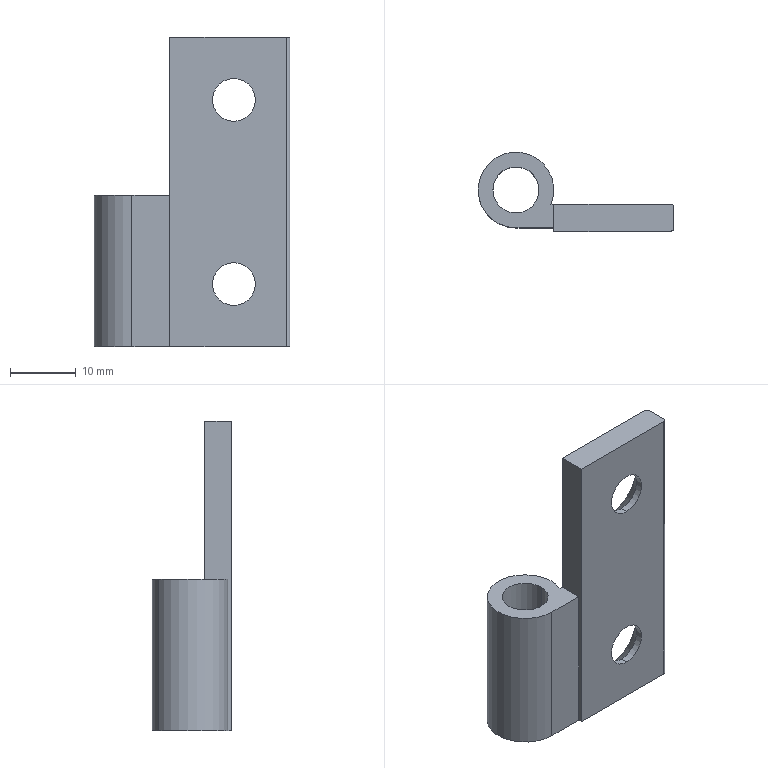Part | SolidWorks | features BaseBody 1 | 1 solid | 22 faces | box 29.75 x 12.05 x 47 mm | volume 4659 mm3 | cylinder 10 | plane 8 | cone 4 | commonest cylinder face diameters 6.5 x4 1 x2 7 x2 11.5 x2
STEP:
#1=CARTESIAN_POINT('',(15.5,1.1,10.75));
#2=VERTEX_POINT('',#1);
#3=CARTESIAN_POINT('',(15.5,1.1,17.25));
#4=VERTEX_POINT('',#3);
#5=CARTESIAN_POINT('',(15.5,1.1,14.));
#6=DIRECTION('',(0.,-1.,0.));
#7=DIRECTION('',(0.,0.,1.));
#8=AXIS2_PLACEMENT_3D('',#5,#6,#7);
#9=CIRCLE('',#8,3.25);
#10=EDGE_CURVE('',#2,#4,#9,.T.);
#11=ORIENTED_EDGE('',*,*,#10,.F.);
#12=CARTESIAN_POINT('',(15.5,0.,10.75));
#13=VERTEX_POINT('',#12);
#14=CARTESIAN_POINT('',(15.5,0.,10.75));
#15=DIRECTION('',(0.,-1.,0.));
#16=VECTOR('',#15,1000.);
#17=LINE('',#14,#16);
#18=EDGE_CURVE('',#2,#13,#17,.T.);
#19=ORIENTED_EDGE('',*,*,#18,.T.);
#20=CARTESIAN_POINT('',(15.5,0.,17.25));
#21=VERTEX_POINT('',#20);
#22=CARTESIAN_POINT('',(15.5,0.,14.));
#23=DIRECTION('',(0.,-1.,0.));
#24=DIRECTION('',(0.,0.,-1.));
#25=AXIS2_PLACEMENT_3D('',#22,#23,#24);
#26=CIRCLE('',#25,3.25);
#27=EDGE_CURVE('',#13,#21,#26,.T.);
#28=ORIENTED_EDGE('',*,*,#27,.T.);
#29=CARTESIAN_POINT('',(15.5,0.,17.25));
#30=DIRECTION('',(0.,-1.,0.));
#31=VECTOR('',#30,1000.);
#32=LINE('',#29,#31);
#33=EDGE_CURVE('',#4,#21,#32,.T.);
#34=ORIENTED_EDGE('',*,*,#33,.F.);
#35=EDGE_LOOP('',(#11,#19,#28,#34));
#36=FACE_OUTER_BOUND('',#35,.T.);
#37=CARTESIAN_POINT('',(15.5,0.,14.));
#38=DIRECTION('',(0.,-1.,0.));
#39=DIRECTION('',(0.000000142,0.,1.));
#40=AXIS2_PLACEMENT_3D('',#37,#38,#39);
#41=CYLINDRICAL_SURFACE('',#40,3.25);
#42=ADVANCED_FACE('',(#36),#41,.F.);
#43=ORIENTED_EDGE('',*,*,#10,.T.);
#44=CARTESIAN_POINT('',(15.5,4.1,20.25));
#45=VERTEX_POINT('',#44);
#46=CARTESIAN_POINT('',(15.5,4.1,20.25));
#47=DIRECTION('',(0.,0.7071,0.7071));
#48=VECTOR('',#47,1000.);
#49=LINE('',#46,#48);
#50=EDGE_CURVE('',#4,#45,#49,.T.);
#51=ORIENTED_EDGE('',*,*,#50,.T.);
#52=CARTESIAN_POINT('',(15.5,4.1,7.75));
#53=VERTEX_POINT('',#52);
#54=CARTESIAN_POINT('',(15.5,4.1,14.));
#55=DIRECTION('',(0.,-1.,0.));
#56=DIRECTION('',(-0.000000001,0.,1.));
#57=AXIS2_PLACEMENT_3D('',#54,#55,#56);
#58=CIRCLE('',#57,6.25);
#59=EDGE_CURVE('',#53,#45,#58,.T.);
#60=ORIENTED_EDGE('',*,*,#59,.F.);
#61=CARTESIAN_POINT('',(15.5,4.1,7.75));
#62=DIRECTION('',(0.,0.7071,-0.7071));
#63=VECTOR('',#62,1000.);
#64=LINE('',#61,#63);
#65=EDGE_CURVE('',#2,#53,#64,.T.);
#66=ORIENTED_EDGE('',*,*,#65,.F.);
#67=EDGE_LOOP('',(#43,#51,#60,#66));
#68=FACE_OUTER_BOUND('',#67,.T.);
#69=CARTESIAN_POINT('',(15.5,4.1,14.));
#70=DIRECTION('',(0.,1.,0.));
#71=DIRECTION('',(0.,0.,-1.));
#72=AXIS2_PLACEMENT_3D('',#69,#70,#71);
#73=CONICAL_SURFACE('',#72,6.25,0.7854);
#74=ADVANCED_FACE('',(#68),#73,.F.);
#75=CARTESIAN_POINT('',(15.5,1.1,-17.25));
#76=VERTEX_POINT('',#75);
#77=CARTESIAN_POINT('',(15.5,1.1,-10.75));
#78=VERTEX_POINT('',#77);
#79=CARTESIAN_POINT('',(15.5,1.1,-14.));
#80=DIRECTION('',(0.,-1.,0.));
#81=DIRECTION('',(0.,0.,1.));
#82=AXIS2_PLACEMENT_3D('',#79,#80,#81);
#83=CIRCLE('',#82,3.25);
#84=EDGE_CURVE('',#76,#78,#83,.T.);
#85=ORIENTED_EDGE('',*,*,#84,.F.);
#86=CARTESIAN_POINT('',(15.5,0.,-17.25));
#87=VERTEX_POINT('',#86);
#88=CARTESIAN_POINT('',(15.5,0.,-17.25));
#89=DIRECTION('',(0.,-1.,0.));
#90=VECTOR('',#89,1000.);
#91=LINE('',#88,#90);
#92=EDGE_CURVE('',#76,#87,#91,.T.);
#93=ORIENTED_EDGE('',*,*,#92,.T.);
#94=CARTESIAN_POINT('',(15.5,0.,-10.75));
#95=VERTEX_POINT('',#94);
#96=CARTESIAN_POINT('',(15.5,0.,-14.));
#97=DIRECTION('',(0.,-1.,0.));
#98=DIRECTION('',(0.,0.,-1.));
#99=AXIS2_PLACEMENT_3D('',#96,#97,#98);
#100=CIRCLE('',#99,3.25);
#101=EDGE_CURVE('',#87,#95,#100,.T.);
#102=ORIENTED_EDGE('',*,*,#101,.T.);
#103=CARTESIAN_POINT('',(15.5,0.,-10.75));
#104=DIRECTION('',(0.,-1.,0.));
#105=VECTOR('',#104,1000.);
#106=LINE('',#103,#105);
#107=EDGE_CURVE('',#78,#95,#106,.T.);
#108=ORIENTED_EDGE('',*,*,#107,.F.);
#109=EDGE_LOOP('',(#85,#93,#102,#108));
#110=FACE_OUTER_BOUND('',#109,.T.);
#111=CARTESIAN_POINT('',(15.5,0.,-14.));
#112=DIRECTION('',(0.,-1.,0.));
#113=DIRECTION('',(0.,0.,1.));
#114=AXIS2_PLACEMENT_3D('',#111,#112,#113);
#115=CYLINDRICAL_SURFACE('',#114,3.25);
#116=ADVANCED_FACE('',(#110),#115,.F.);
#117=ORIENTED_EDGE('',*,*,#84,.T.);
#118=CARTESIAN_POINT('',(15.5,4.1,-7.75));
#119=VERTEX_POINT('',#118);
#120=CARTESIAN_POINT('',(15.5,4.1,-7.75));
#121=DIRECTION('',(0.,0.7071,0.7071));
#122=VECTOR('',#121,1000.);
#123=LINE('',#120,#122);
#124=EDGE_CURVE('',#78,#119,#123,.T.);
#125=ORIENTED_EDGE('',*,*,#124,.T.);
#126=CARTESIAN_POINT('',(15.5,4.1,-20.25));
#127=VERTEX_POINT('',#126);
#128=CARTESIAN_POINT('',(15.5,4.1,-14.));
#129=DIRECTION('',(0.,-1.,0.));
#130=DIRECTION('',(0.,0.,1.));
#131=AXIS2_PLACEMENT_3D('',#128,#129,#130);
#132=CIRCLE('',#131,6.25);
#133=EDGE_CURVE('',#127,#119,#132,.T.);
#134=ORIENTED_EDGE('',*,*,#133,.F.);
#135=CARTESIAN_POINT('',(15.5,4.1,-20.25));
#136=DIRECTION('',(0.,0.7071,-0.7071));
#137=VECTOR('',#136,1000.);
#138=LINE('',#135,#137);
#139=EDGE_CURVE('',#76,#127,#138,.T.);
#140=ORIENTED_EDGE('',*,*,#139,.F.);
#141=EDGE_LOOP('',(#117,#125,#134,#140));
#142=FACE_OUTER_BOUND('',#141,.T.);
#143=CARTESIAN_POINT('',(15.5,4.1,-14.));
#144=DIRECTION('',(0.,1.,0.));
#145=DIRECTION('',(0.,0.,-1.));
#146=AXIS2_PLACEMENT_3D('',#143,#144,#145);
#147=CONICAL_SURFACE('',#146,6.25,0.7854);
#148=ADVANCED_FACE('',(#142),#147,.F.);
#149=CARTESIAN_POINT('',(3.5,6.3,-0.5));
#150=VERTEX_POINT('',#149);
#151=CARTESIAN_POINT('',(-3.5,6.3,-0.5));
#152=VERTEX_POINT('',#151);
#153=CARTESIAN_POINT('',(0.,6.3,-0.5));
#154=DIRECTION('',(0.,0.,1.));
#155=DIRECTION('',(1.,0.,0.));
#156=AXIS2_PLACEMENT_3D('',#153,#154,#155);
#157=CIRCLE('',#156,3.5);
#158=EDGE_CURVE('',#150,#152,#157,.T.);
#159=ORIENTED_EDGE('',*,*,#158,.T.);
#160=CARTESIAN_POINT('',(-3.5,6.3,-23.5));
#161=VERTEX_POINT('',#160);
#162=CARTESIAN_POINT('',(-3.5,6.3,23.5));
#163=DIRECTION('',(0.,0.,-1.));
#164=VECTOR('',#163,1000.);
#165=LINE('',#162,#164);
#166=EDGE_CURVE('',#152,#161,#165,.T.);
#167=ORIENTED_EDGE('',*,*,#166,.T.);
#168=CARTESIAN_POINT('',(3.5,6.3,-23.5));
#169=VERTEX_POINT('',#168);
#170=CARTESIAN_POINT('',(0.,6.3,-23.5));
#171=DIRECTION('',(0.,0.,1.));
#172=DIRECTION('',(-1.,-0.000000142,0.));
#173=AXIS2_PLACEMENT_3D('',#170,#171,#172);
#174=CIRCLE('',#173,3.5);
#175=EDGE_CURVE('',#169,#161,#174,.T.);
#176=ORIENTED_EDGE('',*,*,#175,.F.);
#177=CARTESIAN_POINT('',(3.5,6.3,23.5));
#178=DIRECTION('',(0.,0.,-1.));
#179=VECTOR('',#178,1000.);
#180=LINE('',#177,#179);
#181=EDGE_CURVE('',#150,#169,#180,.T.);
#182=ORIENTED_EDGE('',*,*,#181,.F.);
#183=EDGE_LOOP('',(#159,#167,#176,#182));
#184=FACE_OUTER_BOUND('',#183,.T.);
#185=CARTESIAN_POINT('',(0.,6.3,23.5));
#186=DIRECTION('',(0.,0.,-1.));
#187=DIRECTION('',(1.,0.,0.));
#188=AXIS2_PLACEMENT_3D('',#185,#186,#187);
#189=CYLINDRICAL_SURFACE('',#188,3.5);
#190=ADVANCED_FACE('',(#184),#189,.F.);
#191=CARTESIAN_POINT('',(-3.195,11.081,-0.5));
#192=VERTEX_POINT('',#191);
#193=CARTESIAN_POINT('',(0.,0.55,-0.5));
#194=VERTEX_POINT('',#193);
#195=CARTESIAN_POINT('',(0.,6.3,-0.5));
#196=DIRECTION('',(0.,0.,1.));
#197=DIRECTION('',(0.,-1.,0.));
#198=AXIS2_PLACEMENT_3D('',#195,#196,#197);
#199=CIRCLE('',#198,5.75);
#200=EDGE_CURVE('',#192,#194,#199,.T.);
#201=ORIENTED_EDGE('',*,*,#200,.F.);
#202=CARTESIAN_POINT('',(-3.195,11.081,-23.5));
#203=VERTEX_POINT('',#202);
#204=CARTESIAN_POINT('',(-3.195,11.081,23.5));
#205=DIRECTION('',(0.,0.,-1.));
#206=VECTOR('',#205,1000.);
#207=LINE('',#204,#206);
#208=EDGE_CURVE('',#192,#203,#207,.T.);
#209=ORIENTED_EDGE('',*,*,#208,.T.);
#210=CARTESIAN_POINT('',(0.,0.55,-23.5));
#211=VERTEX_POINT('',#210);
#212=CARTESIAN_POINT('',(0.,6.3,-23.5));
#213=DIRECTION('',(0.,0.,1.));
#214=DIRECTION('',(0.9239,-0.3826,0.));
#215=AXIS2_PLACEMENT_3D('',#212,#213,#214);
#216=CIRCLE('',#215,5.75);
#217=EDGE_CURVE('',#203,#211,#216,.T.);
#218=ORIENTED_EDGE('',*,*,#217,.T.);
#219=CARTESIAN_POINT('',(0.,0.55,-23.5));
#220=DIRECTION('',(0.,0.,-1.));
#221=VECTOR('',#220,1000.);
#222=LINE('',#219,#221);
#223=EDGE_CURVE('',#194,#211,#222,.T.);
#224=ORIENTED_EDGE('',*,*,#223,.F.);
#225=EDGE_LOOP('',(#201,#209,#218,#224));
#226=FACE_OUTER_BOUND('',#225,.T.);
#227=CARTESIAN_POINT('',(0.,6.3,23.5));
#228=DIRECTION('',(0.,0.,-1.));
#229=DIRECTION('',(-0.5556,0.8314,0.));
#230=AXIS2_PLACEMENT_3D('',#227,#228,#229);
#231=CYLINDRICAL_SURFACE('',#230,5.75);
#232=ADVANCED_FACE('',(#226),#231,.T.);
#233=CARTESIAN_POINT('',(5.75,4.1,23.5));
#234=VERTEX_POINT('',#233);
#235=CARTESIAN_POINT('',(5.75,4.1,-0.5));
#236=VERTEX_POINT('',#235);
#237=CARTESIAN_POINT('',(5.75,4.1,-0.5));
#238=DIRECTION('',(0.,0.,-1.));
#239=VECTOR('',#238,1000.);
#240=LINE('',#237,#239);
#241=EDGE_CURVE('',#234,#236,#240,.T.);
#242=ORIENTED_EDGE('',*,*,#241,.F.);
#243=CARTESIAN_POINT('',(23.5,4.1,23.5));
#244=VERTEX_POINT('',#243);
#245=CARTESIAN_POINT('',(5.75,4.1,23.5));
#246=DIRECTION('',(-1.,0.,0.));
#247=VECTOR('',#246,1000.);
#248=LINE('',#245,#247);
#249=EDGE_CURVE('',#244,#234,#248,.T.);
#250=ORIENTED_EDGE('',*,*,#249,.F.);
#251=CARTESIAN_POINT('',(23.5,4.1,-23.5));
#252=VERTEX_POINT('',#251);
#253=CARTESIAN_POINT('',(23.5,4.1,23.5));
#254=DIRECTION('',(0.,0.,-1.));
#255=VECTOR('',#254,1000.);
#256=LINE('',#253,#255);
#257=EDGE_CURVE('',#244,#252,#256,.T.);
#258=ORIENTED_EDGE('',*,*,#257,.T.);
#259=CARTESIAN_POINT('',(5.312,4.1,-23.5));
#260=VERTEX_POINT('',#259);
#261=CARTESIAN_POINT('',(23.5,4.1,-23.5));
#262=DIRECTION('',(-1.,0.,0.));
#263=VECTOR('',#262,1000.);
#264=LINE('',#261,#263);
#265=EDGE_CURVE('',#252,#260,#264,.T.);
#266=ORIENTED_EDGE('',*,*,#265,.T.);
#267=CARTESIAN_POINT('',(5.312,4.1,-0.5));
#268=VERTEX_POINT('',#267);
#269=CARTESIAN_POINT('',(5.312,4.1,-23.5));
#270=DIRECTION('',(0.,0.,-1.));
#271=VECTOR('',#270,1000.);
#272=LINE('',#269,#271);
#273=EDGE_CURVE('',#268,#260,#272,.T.);
#274=ORIENTED_EDGE('',*,*,#273,.F.);
#275=CARTESIAN_POINT('',(5.312,4.1,-0.5));
#276=DIRECTION('',(-1.,0.,0.));
#277=VECTOR('',#276,1000.);
#278=LINE('',#275,#277);
#279=EDGE_CURVE('',#236,#268,#278,.T.);
#280=ORIENTED_EDGE('',*,*,#279,.F.);
#281=EDGE_LOOP('',(#242,#250,#258,#266,#274,#280));
#282=FACE_OUTER_BOUND('',#281,.T.);
#283=ORIENTED_EDGE('',*,*,#133,.T.);
#284=CARTESIAN_POINT('',(15.5,4.1,-14.));
#285=DIRECTION('',(0.,-1.,0.));
#286=DIRECTION('',(0.,0.,1.));
#287=AXIS2_PLACEMENT_3D('',#284,#285,#286);
#288=CIRCLE('',#287,6.25);
#289=EDGE_CURVE('',#119,#127,#288,.T.);
#290=ORIENTED_EDGE('',*,*,#289,.T.);
#291=EDGE_LOOP('',(#283,#290));
#292=FACE_BOUND('',#291,.T.);
#293=ORIENTED_EDGE('',*,*,#59,.T.);
#294=CARTESIAN_POINT('',(15.5,4.1,14.));
#295=DIRECTION('',(0.,-1.,0.));
#296=DIRECTION('',(-0.000000001,0.,1.));
#297=AXIS2_PLACEMENT_3D('',#294,#295,#296);
#298=CIRCLE('',#297,6.25);
#299=EDGE_CURVE('',#45,#53,#298,.T.);
#300=ORIENTED_EDGE('',*,*,#299,.T.);
#301=EDGE_LOOP('',(#293,#300));
#302=FACE_BOUND('',#301,.T.);
#303=CARTESIAN_POINT('',(5.312,4.1,23.5));
#304=DIRECTION('',(0.,1.,0.));
#305=DIRECTION('',(1.,0.,0.));
#306=AXIS2_PLACEMENT_3D('',#303,#304,#305);
#307=PLANE('',#306);
#308=ADVANCED_FACE('',(#282,#292,#302),#307,.T.);
#309=ORIENTED_EDGE('',*,*,#208,.F.);
#310=CARTESIAN_POINT('',(0.,6.3,-0.5));
#311=DIRECTION('',(0.,0.,1.));
#312=DIRECTION('',(0.,-1.,0.));
#313=AXIS2_PLACEMENT_3D('',#310,#311,#312);
#314=CIRCLE('',#313,5.75);
#315=EDGE_CURVE('',#268,#192,#314,.T.);
#316=ORIENTED_EDGE('',*,*,#315,.F.);
#317=ORIENTED_EDGE('',*,*,#273,.T.);
#318=CARTESIAN_POINT('',(0.,6.3,-23.5));
#319=DIRECTION('',(0.,0.,1.));
#320=DIRECTION('',(0.9239,-0.3826,0.));
#321=AXIS2_PLACEMENT_3D('',#318,#319,#320);
#322=CIRCLE('',#321,5.75);
#323=EDGE_CURVE('',#260,#203,#322,.T.);
#324=ORIENTED_EDGE('',*,*,#323,.T.);
#325=EDGE_LOOP('',(#309,#316,#317,#324));
#326=FACE_OUTER_BOUND('',#325,.T.);
#327=CARTESIAN_POINT('',(0.,6.3,23.5));
#328=DIRECTION('',(0.,0.,-1.));
#329=DIRECTION('',(-0.5556,0.8314,0.));
#330=AXIS2_PLACEMENT_3D('',#327,#328,#329);
#331=CYLINDRICAL_SURFACE('',#330,5.75);
#332=ADVANCED_FACE('',(#326),#331,.T.);
#333=CARTESIAN_POINT('',(5.75,0.55,-0.5));
#334=VERTEX_POINT('',#333);
#335=CARTESIAN_POINT('',(5.75,0.55,-0.5));
#336=DIRECTION('',(1.,0.,0.));
#337=VECTOR('',#336,1000.);
#338=LINE('',#335,#337);
#339=EDGE_CURVE('',#194,#334,#338,.T.);
#340=ORIENTED_EDGE('',*,*,#339,.F.);
#341=ORIENTED_EDGE('',*,*,#223,.T.);
#342=CARTESIAN_POINT('',(5.75,0.55,-23.5));
#343=VERTEX_POINT('',#342);
#344=CARTESIAN_POINT('',(0.,0.55,-23.5));
#345=DIRECTION('',(1.,0.,0.));
#346=VECTOR('',#345,1000.);
#347=LINE('',#344,#346);
#348=EDGE_CURVE('',#211,#343,#347,.T.);
#349=ORIENTED_EDGE('',*,*,#348,.T.);
#350=CARTESIAN_POINT('',(5.75,0.55,-23.5));
#351=DIRECTION('',(0.,0.,-1.));
#352=VECTOR('',#351,1000.);
#353=LINE('',#350,#352);
#354=EDGE_CURVE('',#334,#343,#353,.T.);
#355=ORIENTED_EDGE('',*,*,#354,.F.);
#356=EDGE_LOOP('',(#340,#341,#349,#355));
#357=FACE_OUTER_BOUND('',#356,.T.);
#358=CARTESIAN_POINT('',(0.,0.55,-23.5));
#359=DIRECTION('',(0.,-1.,0.));
#360=DIRECTION('',(1.,0.,0.));
#361=AXIS2_PLACEMENT_3D('',#358,#359,#360);
#362=PLANE('',#361);
#363=ADVANCED_FACE('',(#357),#362,.T.);
#364=ORIENTED_EDGE('',*,*,#249,.T.);
#365=CARTESIAN_POINT('',(5.75,0.,23.5));
#366=VERTEX_POINT('',#365);
#367=CARTESIAN_POINT('',(5.75,4.1,23.5));
#368=DIRECTION('',(0.,-1.,0.));
#369=VECTOR('',#368,1000.);
#370=LINE('',#367,#369);
#371=EDGE_CURVE('',#234,#366,#370,.T.);
#372=ORIENTED_EDGE('',*,*,#371,.T.);
#373=CARTESIAN_POINT('',(23.5,0.,23.5));
#374=VERTEX_POINT('',#373);
#375=CARTESIAN_POINT('',(5.75,0.,23.5));
#376=DIRECTION('',(1.,0.,0.));
#377=VECTOR('',#376,1000.);
#378=LINE('',#375,#377);
#379=EDGE_CURVE('',#366,#374,#378,.T.);
#380=ORIENTED_EDGE('',*,*,#379,.T.);
#381=CARTESIAN_POINT('',(24.,0.5,23.5));
#382=VERTEX_POINT('',#381);
#383=CARTESIAN_POINT('',(23.5,0.5,23.5));
#384=DIRECTION('',(0.,0.,1.));
#385=DIRECTION('',(0.,-1.,0.));
#386=AXIS2_PLACEMENT_3D('',#383,#384,#385);
#387=CIRCLE('',#386,0.5);
#388=EDGE_CURVE('',#374,#382,#387,.T.);
#389=ORIENTED_EDGE('',*,*,#388,.T.);
#390=CARTESIAN_POINT('',(24.,3.6,23.5));
#391=VERTEX_POINT('',#390);
#392=CARTESIAN_POINT('',(24.,0.5,23.5));
#393=DIRECTION('',(0.,1.,0.));
#394=VECTOR('',#393,1000.);
#395=LINE('',#392,#394);
#396=EDGE_CURVE('',#382,#391,#395,.T.);
#397=ORIENTED_EDGE('',*,*,#396,.T.);
#398=CARTESIAN_POINT('',(23.5,3.6,23.5));
#399=DIRECTION('',(0.,0.,1.));
#400=DIRECTION('',(1.,0.,0.));
#401=AXIS2_PLACEMENT_3D('',#398,#399,#400);
#402=CIRCLE('',#401,0.5);
#403=EDGE_CURVE('',#391,#244,#402,.T.);
#404=ORIENTED_EDGE('',*,*,#403,.T.);
#405=EDGE_LOOP('',(#364,#372,#380,#389,#397,#404));
#406=FACE_OUTER_BOUND('',#405,.T.);
#407=CARTESIAN_POINT('',(5.75,0.,23.5));
#408=DIRECTION('',(0.,0.,1.));
#409=DIRECTION('',(1.,0.,0.));
#410=AXIS2_PLACEMENT_3D('',#407,#408,#409);
#411=PLANE('',#410);
#412=ADVANCED_FACE('',(#406),#411,.T.);
#413=ORIENTED_EDGE('',*,*,#371,.F.);
#414=ORIENTED_EDGE('',*,*,#241,.T.);
#415=CARTESIAN_POINT('',(5.75,4.1,-0.5));
#416=DIRECTION('',(0.,-1.,0.));
#417=VECTOR('',#416,1000.);
#418=LINE('',#415,#417);
#419=EDGE_CURVE('',#236,#334,#418,.T.);
#420=ORIENTED_EDGE('',*,*,#419,.T.);
#421=ORIENTED_EDGE('',*,*,#354,.T.);
#422=CARTESIAN_POINT('',(5.75,0.,-23.5));
#423=VERTEX_POINT('',#422);
#424=CARTESIAN_POINT('',(5.75,0.55,-23.5));
#425=DIRECTION('',(0.,-1.,0.));
#426=VECTOR('',#425,1000.);
#427=LINE('',#424,#426);
#428=EDGE_CURVE('',#343,#423,#427,.T.);
#429=ORIENTED_EDGE('',*,*,#428,.T.);
#430=CARTESIAN_POINT('',(5.75,0.,-23.5));
#431=DIRECTION('',(0.,0.,-1.));
#432=VECTOR('',#431,1000.);
#433=LINE('',#430,#432);
#434=EDGE_CURVE('',#366,#423,#433,.T.);
#435=ORIENTED_EDGE('',*,*,#434,.F.);
#436=EDGE_LOOP('',(#413,#414,#420,#421,#429,#435));
#437=FACE_OUTER_BOUND('',#436,.T.);
#438=CARTESIAN_POINT('',(5.75,0.,23.5));
#439=DIRECTION('',(-1.,0.,0.));
#440=DIRECTION('',(0.,1.,0.));
#441=AXIS2_PLACEMENT_3D('',#438,#439,#440);
#442=PLANE('',#441);
#443=ADVANCED_FACE('',(#437),#442,.T.);
#444=CARTESIAN_POINT('',(23.5,0.,-23.5));
#445=VERTEX_POINT('',#444);
#446=CARTESIAN_POINT('',(5.75,0.,-23.5));
#447=DIRECTION('',(1.,0.,0.));
#448=VECTOR('',#447,1000.);
#449=LINE('',#446,#448);
#450=EDGE_CURVE('',#423,#445,#449,.T.);
#451=ORIENTED_EDGE('',*,*,#450,.T.);
#452=CARTESIAN_POINT('',(23.5,0.,-23.5));
#453=DIRECTION('',(0.,0.,-1.));
#454=VECTOR('',#453,1000.);
#455=LINE('',#452,#454);
#456=EDGE_CURVE('',#374,#445,#455,.T.);
#457=ORIENTED_EDGE('',*,*,#456,.F.);
#458=ORIENTED_EDGE('',*,*,#379,.F.);
#459=ORIENTED_EDGE('',*,*,#434,.T.);
#460=EDGE_LOOP('',(#451,#457,#458,#459));
#461=FACE_OUTER_BOUND('',#460,.T.);
#462=CARTESIAN_POINT('',(15.5,0.,-14.));
#463=DIRECTION('',(0.,-1.,0.));
#464=DIRECTION('',(0.,0.,-1.));
#465=AXIS2_PLACEMENT_3D('',#462,#463,#464);
#466=CIRCLE('',#465,3.25);
#467=EDGE_CURVE('',#95,#87,#466,.T.);
#468=ORIENTED_EDGE('',*,*,#467,.F.);
#469=ORIENTED_EDGE('',*,*,#101,.F.);
#470=EDGE_LOOP('',(#468,#469));
#471=FACE_BOUND('',#470,.T.);
#472=CARTESIAN_POINT('',(15.5,0.,14.));
#473=DIRECTION('',(0.,-1.,0.));
#474=DIRECTION('',(0.,0.,-1.));
#475=AXIS2_PLACEMENT_3D('',#472,#473,#474);
#476=CIRCLE('',#475,3.25);
#477=EDGE_CURVE('',#21,#13,#476,.T.);
#478=ORIENTED_EDGE('',*,*,#477,.F.);
#479=ORIENTED_EDGE('',*,*,#27,.F.);
#480=EDGE_LOOP('',(#478,#479));
#481=FACE_BOUND('',#480,.T.);
#482=CARTESIAN_POINT('',(5.75,0.,-23.5));
#483=DIRECTION('',(0.,-1.,0.));
#484=DIRECTION('',(1.,0.,0.));
#485=AXIS2_PLACEMENT_3D('',#482,#483,#484);
#486=PLANE('',#485);
#487=ADVANCED_FACE('',(#461,#471,#481),#486,.T.);
#488=CARTESIAN_POINT('',(24.,0.5,-23.5));
#489=VERTEX_POINT('',#488);
#490=CARTESIAN_POINT('',(23.5,0.5,-23.5));
#491=DIRECTION('',(0.,0.,1.));
#492=DIRECTION('',(0.,-1.,0.));
#493=AXIS2_PLACEMENT_3D('',#490,#491,#492);
#494=CIRCLE('',#493,0.5);
#495=EDGE_CURVE('',#445,#489,#494,.T.);
#496=ORIENTED_EDGE('',*,*,#495,.T.);
#497=CARTESIAN_POINT('',(24.,0.5,-23.5));
#498=DIRECTION('',(0.,0.,-1.));
#499=VECTOR('',#498,1000.);
#500=LINE('',#497,#499);
#501=EDGE_CURVE('',#382,#489,#500,.T.);
#502=ORIENTED_EDGE('',*,*,#501,.F.);
#503=ORIENTED_EDGE('',*,*,#388,.F.);
#504=ORIENTED_EDGE('',*,*,#456,.T.);
#505=EDGE_LOOP('',(#496,#502,#503,#504));
#506=FACE_OUTER_BOUND('',#505,.T.);
#507=CARTESIAN_POINT('',(23.5,0.5,23.5));
#508=DIRECTION('',(0.,0.,-1.));
#509=DIRECTION('',(1.,0.,0.));
#510=AXIS2_PLACEMENT_3D('',#507,#508,#509);
#511=CYLINDRICAL_SURFACE('',#510,0.5);
#512=ADVANCED_FACE('',(#506),#511,.T.);
#513=CARTESIAN_POINT('',(24.,3.6,-23.5));
#514=VERTEX_POINT('',#513);
#515=CARTESIAN_POINT('',(24.,0.5,-23.5));
#516=DIRECTION('',(0.,1.,0.));
#517=VECTOR('',#516,1000.);
#518=LINE('',#515,#517);
#519=EDGE_CURVE('',#489,#514,#518,.T.);
#520=ORIENTED_EDGE('',*,*,#519,.T.);
#521=CARTESIAN_POINT('',(24.,3.6,-23.5));
#522=DIRECTION('',(0.,0.,-1.));
#523=VECTOR('',#522,1000.);
#524=LINE('',#521,#523);
#525=EDGE_CURVE('',#391,#514,#524,.T.);
#526=ORIENTED_EDGE('',*,*,#525,.F.);
#527=ORIENTED_EDGE('',*,*,#396,.F.);
#528=ORIENTED_EDGE('',*,*,#501,.T.);
#529=EDGE_LOOP('',(#520,#526,#527,#528));
#530=FACE_OUTER_BOUND('',#529,.T.);
#531=CARTESIAN_POINT('',(24.,0.5,-23.5));
#532=DIRECTION('',(1.,0.,0.));
#533=DIRECTION('',(0.,1.,0.));
#534=AXIS2_PLACEMENT_3D('',#531,#532,#533);
#535=PLANE('',#534);
#536=ADVANCED_FACE('',(#530),#535,.T.);
#537=CARTESIAN_POINT('',(23.5,3.6,-23.5));
#538=DIRECTION('',(0.,0.,1.));
#539=DIRECTION('',(1.,0.,0.));
#540=AXIS2_PLACEMENT_3D('',#537,#538,#539);
#541=CIRCLE('',#540,0.5);
#542=EDGE_CURVE('',#514,#252,#541,.T.);
#543=ORIENTED_EDGE('',*,*,#542,.T.);
#544=ORIENTED_EDGE('',*,*,#257,.F.);
#545=ORIENTED_EDGE('',*,*,#403,.F.);
#546=ORIENTED_EDGE('',*,*,#525,.T.);
#547=EDGE_LOOP('',(#543,#544,#545,#546));
#548=FACE_OUTER_BOUND('',#547,.T.);
#549=CARTESIAN_POINT('',(23.5,3.6,23.5));
#550=DIRECTION('',(0.,0.,-1.));
#551=DIRECTION('',(0.,1.,0.));
#552=AXIS2_PLACEMENT_3D('',#549,#550,#551);
#553=CYLINDRICAL_SURFACE('',#552,0.5);
#554=ADVANCED_FACE('',(#548),#553,.T.);
#555=ORIENTED_EDGE('',*,*,#323,.F.);
#556=ORIENTED_EDGE('',*,*,#265,.F.);
#557=ORIENTED_EDGE('',*,*,#542,.F.);
#558=ORIENTED_EDGE('',*,*,#519,.F.);
#559=ORIENTED_EDGE('',*,*,#495,.F.);
#560=ORIENTED_EDGE('',*,*,#450,.F.);
#561=ORIENTED_EDGE('',*,*,#428,.F.);
#562=ORIENTED_EDGE('',*,*,#348,.F.);
#563=ORIENTED_EDGE('',*,*,#217,.F.);
#564=EDGE_LOOP('',(#555,#556,#557,#558,#559,#560,#561,#562,#563));
#565=FACE_OUTER_BOUND('',#564,.T.);
#566=ORIENTED_EDGE('',*,*,#175,.T.);
#567=CARTESIAN_POINT('',(0.,6.3,-23.5));
#568=DIRECTION('',(0.,0.,1.));
#569=DIRECTION('',(-1.,-0.000000142,0.));
#570=AXIS2_PLACEMENT_3D('',#567,#568,#569);
#571=CIRCLE('',#570,3.5);
#572=EDGE_CURVE('',#161,#169,#571,.T.);
#573=ORIENTED_EDGE('',*,*,#572,.T.);
#574=EDGE_LOOP('',(#566,#573));
#575=FACE_BOUND('',#574,.T.);
#576=CARTESIAN_POINT('',(-6.305,0.,-23.5));
#577=DIRECTION('',(0.,0.,-1.));
#578=DIRECTION('',(0.,1.,0.));
#579=AXIS2_PLACEMENT_3D('',#576,#577,#578);
#580=PLANE('',#579);
#581=ADVANCED_FACE('',(#565,#575),#580,.T.);
#582=ORIENTED_EDGE('',*,*,#279,.T.);
#583=ORIENTED_EDGE('',*,*,#315,.T.);
#584=ORIENTED_EDGE('',*,*,#200,.T.);
#585=ORIENTED_EDGE('',*,*,#339,.T.);
#586=ORIENTED_EDGE('',*,*,#419,.F.);
#587=EDGE_LOOP('',(#582,#583,#584,#585,#586));
#588=FACE_OUTER_BOUND('',#587,.T.);
#589=ORIENTED_EDGE('',*,*,#158,.F.);
#590=CARTESIAN_POINT('',(0.,6.3,-0.5));
#591=DIRECTION('',(0.,0.,1.));
#592=DIRECTION('',(1.,0.,0.));
#593=AXIS2_PLACEMENT_3D('',#590,#591,#592);
#594=CIRCLE('',#593,3.5);
#595=EDGE_CURVE('',#152,#150,#594,.T.);
#596=ORIENTED_EDGE('',*,*,#595,.F.);
#597=EDGE_LOOP('',(#589,#596));
#598=FACE_BOUND('',#597,.T.);
#599=CARTESIAN_POINT('',(-5.849,0.55,-0.5));
#600=DIRECTION('',(0.,0.,1.));
#601=DIRECTION('',(1.,0.,0.));
#602=AXIS2_PLACEMENT_3D('',#599,#600,#601);
#603=PLANE('',#602);
#604=ADVANCED_FACE('',(#588,#598),#603,.T.);
#605=ORIENTED_EDGE('',*,*,#166,.F.);
#606=ORIENTED_EDGE('',*,*,#595,.T.);
#607=ORIENTED_EDGE('',*,*,#181,.T.);
#608=ORIENTED_EDGE('',*,*,#572,.F.);
#609=EDGE_LOOP('',(#605,#606,#607,#608));
#610=FACE_OUTER_BOUND('',#609,.T.);
#611=CARTESIAN_POINT('',(0.,6.3,23.5));
#612=DIRECTION('',(0.,0.,-1.));
#613=DIRECTION('',(1.,0.,0.));
#614=AXIS2_PLACEMENT_3D('',#611,#612,#613);
#615=CYLINDRICAL_SURFACE('',#614,3.5);
#616=ADVANCED_FACE('',(#610),#615,.F.);
#617=ORIENTED_EDGE('',*,*,#124,.F.);
#618=CARTESIAN_POINT('',(15.5,1.1,-14.));
#619=DIRECTION('',(0.,-1.,0.));
#620=DIRECTION('',(0.,0.,1.));
#621=AXIS2_PLACEMENT_3D('',#618,#619,#620);
#622=CIRCLE('',#621,3.25);
#623=EDGE_CURVE('',#78,#76,#622,.T.);
#624=ORIENTED_EDGE('',*,*,#623,.T.);
#625=ORIENTED_EDGE('',*,*,#139,.T.);
#626=ORIENTED_EDGE('',*,*,#289,.F.);
#627=EDGE_LOOP('',(#617,#624,#625,#626));
#628=FACE_OUTER_BOUND('',#627,.T.);
#629=CARTESIAN_POINT('',(15.5,4.1,-14.));
#630=DIRECTION('',(0.,1.,0.));
#631=DIRECTION('',(0.,0.,-1.));
#632=AXIS2_PLACEMENT_3D('',#629,#630,#631);
#633=CONICAL_SURFACE('',#632,6.25,0.7854);
#634=ADVANCED_FACE('',(#628),#633,.F.);
#635=ORIENTED_EDGE('',*,*,#92,.F.);
#636=ORIENTED_EDGE('',*,*,#623,.F.);
#637=ORIENTED_EDGE('',*,*,#107,.T.);
#638=ORIENTED_EDGE('',*,*,#467,.T.);
#639=EDGE_LOOP('',(#635,#636,#637,#638));
#640=FACE_OUTER_BOUND('',#639,.T.);
#641=CARTESIAN_POINT('',(15.5,0.,-14.));
#642=DIRECTION('',(0.,-1.,0.));
#643=DIRECTION('',(0.,0.,1.));
#644=AXIS2_PLACEMENT_3D('',#641,#642,#643);
#645=CYLINDRICAL_SURFACE('',#644,3.25);
#646=ADVANCED_FACE('',(#640),#645,.F.);
#647=ORIENTED_EDGE('',*,*,#50,.F.);
#648=CARTESIAN_POINT('',(15.5,1.1,14.));
#649=DIRECTION('',(0.,-1.,0.));
#650=DIRECTION('',(0.,0.,1.));
#651=AXIS2_PLACEMENT_3D('',#648,#649,#650);
#652=CIRCLE('',#651,3.25);
#653=EDGE_CURVE('',#4,#2,#652,.T.);
#654=ORIENTED_EDGE('',*,*,#653,.T.);
#655=ORIENTED_EDGE('',*,*,#65,.T.);
#656=ORIENTED_EDGE('',*,*,#299,.F.);
#657=EDGE_LOOP('',(#647,#654,#655,#656));
#658=FACE_OUTER_BOUND('',#657,.T.);
#659=CARTESIAN_POINT('',(15.5,4.1,14.));
#660=DIRECTION('',(0.,1.,0.));
#661=DIRECTION('',(0.,0.,-1.));
#662=AXIS2_PLACEMENT_3D('',#659,#660,#661);
#663=CONICAL_SURFACE('',#662,6.25,0.7854);
#664=ADVANCED_FACE('',(#658),#663,.F.);
#665=ORIENTED_EDGE('',*,*,#18,.F.);
#666=ORIENTED_EDGE('',*,*,#653,.F.);
#667=ORIENTED_EDGE('',*,*,#33,.T.);
#668=ORIENTED_EDGE('',*,*,#477,.T.);
#669=EDGE_LOOP('',(#665,#666,#667,#668));
#670=FACE_OUTER_BOUND('',#669,.T.);
#671=CARTESIAN_POINT('',(15.5,0.,14.));
#672=DIRECTION('',(0.,-1.,0.));
#673=DIRECTION('',(0.000000142,0.,1.));
#674=AXIS2_PLACEMENT_3D('',#671,#672,#673);
#675=CYLINDRICAL_SURFACE('',#674,3.25);
#676=ADVANCED_FACE('',(#670),#675,.F.);
#677=CLOSED_SHELL('',(#42,#74,#116,#148,#190,#232,#308,#332,#363,#412,#443,#487,#512,#536,#554,#581,#604,#616,#634,#646,#664,#676));
#678=MANIFOLD_SOLID_BREP('',#677);
#679=CARTESIAN_POINT('',(0.,0.,0.));
#680=DIRECTION('',(0.,0.,1.));
#681=DIRECTION('',(1.,0.,0.));
#682=AXIS2_PLACEMENT_3D('',#679,#680,#681);
#683=(LENGTH_UNIT()NAMED_UNIT(*)SI_UNIT(.MILLI.,.METRE.));
#684=UNCERTAINTY_MEASURE_WITH_UNIT(LENGTH_MEASURE(0.00001),#683,'','');
#685=(NAMED_UNIT(*)PLANE_ANGLE_UNIT()SI_UNIT($,.RADIAN.));
#686=(NAMED_UNIT(*)SI_UNIT($,.STERADIAN.)SOLID_ANGLE_UNIT());
#687=(GEOMETRIC_REPRESENTATION_CONTEXT(3)GLOBAL_UNCERTAINTY_ASSIGNED_CONTEXT((#684))GLOBAL_UNIT_ASSIGNED_CONTEXT((#683,#685,#686))REPRESENTATION_CONTEXT('',''));
#688=ADVANCED_BREP_SHAPE_REPRESENTATION('',(#678,#682),#687);